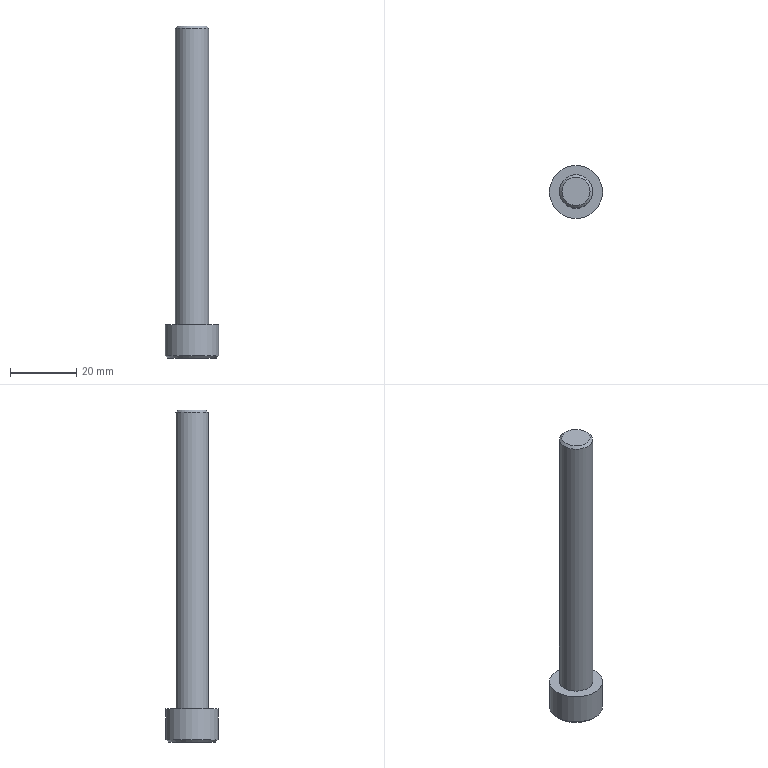Part | STEP file | M10.00-90.00 | 1 solid | 14 faces | box 16 x 16 x 100 mm | volume 8744 mm3 | plane 10 | cylinder 2 | cone 2 | commonest cylinder face diameters 10 x1 16 x1